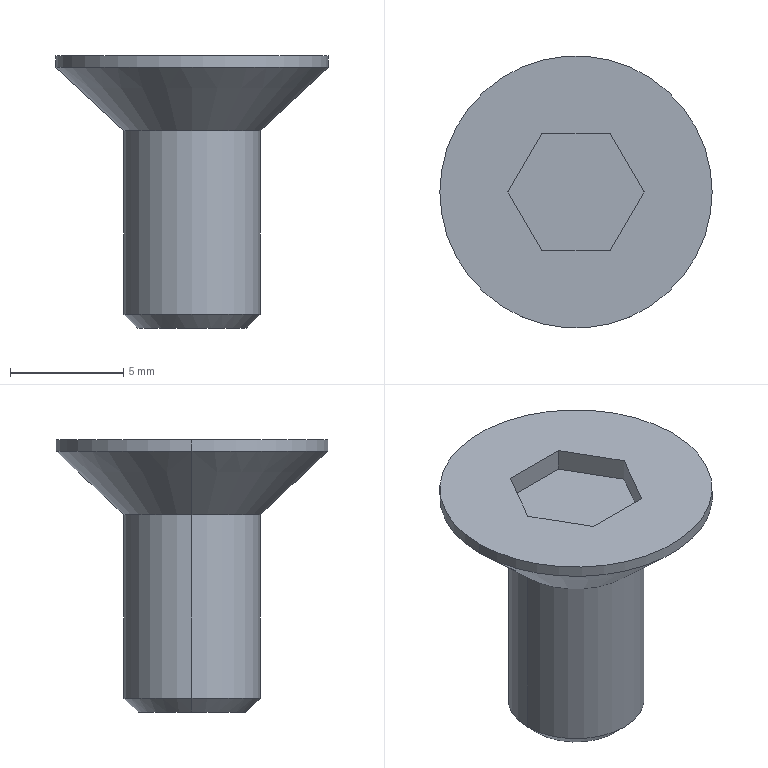Part | SolidWorks | features Chamfer 1, ICE 1, Revolution 1 | 1 solid | 17 faces | box 12 x 12 x 12 mm | volume 460.573 mm3 | plane 9 | cone 4 | cylinder 4 | commonest cylinder face diameters 6 x2 12 x2
STEP:
#1=CARTESIAN_POINT('',(-2.386,0.,-12.));
#2=VERTEX_POINT('',#1);
#3=CARTESIAN_POINT('',(2.386,0.,-12.));
#4=VERTEX_POINT('',#3);
#5=CARTESIAN_POINT('',(0.,0.,-12.));
#6=DIRECTION('',(0.,0.,-1.));
#7=DIRECTION('',(-1.,0.,0.));
#8=AXIS2_PLACEMENT_3D('',#5,#6,#7);
#9=CIRCLE('',#8,2.386);
#10=EDGE_CURVE('',#2,#4,#9,.T.);
#11=ORIENTED_EDGE('',*,*,#10,.F.);
#12=CARTESIAN_POINT('',(-3.,0.,-11.387));
#13=VERTEX_POINT('',#12);
#14=CARTESIAN_POINT('',(-3.,0.,-11.387));
#15=DIRECTION('',(-0.7071,0.,0.7071));
#16=VECTOR('',#15,1000.);
#17=LINE('',#14,#16);
#18=EDGE_CURVE('',#2,#13,#17,.T.);
#19=ORIENTED_EDGE('',*,*,#18,.T.);
#20=CARTESIAN_POINT('',(3.,0.,-11.387));
#21=VERTEX_POINT('',#20);
#22=CARTESIAN_POINT('',(0.,0.,-11.387));
#23=DIRECTION('',(0.,0.,1.));
#24=DIRECTION('',(-1.,0.,0.));
#25=AXIS2_PLACEMENT_3D('',#22,#23,#24);
#26=CIRCLE('',#25,3.);
#27=EDGE_CURVE('',#21,#13,#26,.T.);
#28=ORIENTED_EDGE('',*,*,#27,.F.);
#29=CARTESIAN_POINT('',(3.,0.,-11.387));
#30=DIRECTION('',(0.7071,0.,0.7071));
#31=VECTOR('',#30,1000.);
#32=LINE('',#29,#31);
#33=EDGE_CURVE('',#4,#21,#32,.T.);
#34=ORIENTED_EDGE('',*,*,#33,.F.);
#35=EDGE_LOOP('',(#11,#19,#28,#34));
#36=FACE_OUTER_BOUND('',#35,.T.);
#37=CARTESIAN_POINT('',(0.,0.,-11.387));
#38=DIRECTION('',(0.,0.,1.));
#39=DIRECTION('',(1.,0.,0.));
#40=AXIS2_PLACEMENT_3D('',#37,#38,#39);
#41=CONICAL_SURFACE('',#40,3.,0.7854);
#42=ADVANCED_FACE('',(#36),#41,.T.);
#43=CARTESIAN_POINT('',(3.,0.,-3.3));
#44=VERTEX_POINT('',#43);
#45=CARTESIAN_POINT('',(-3.,0.,-3.3));
#46=VERTEX_POINT('',#45);
#47=CARTESIAN_POINT('',(0.,0.,-3.3));
#48=DIRECTION('',(0.,0.,1.));
#49=DIRECTION('',(1.,0.,0.));
#50=AXIS2_PLACEMENT_3D('',#47,#48,#49);
#51=CIRCLE('',#50,3.);
#52=EDGE_CURVE('',#44,#46,#51,.T.);
#53=ORIENTED_EDGE('',*,*,#52,.T.);
#54=CARTESIAN_POINT('',(-6.,0.,-0.5));
#55=VERTEX_POINT('',#54);
#56=CARTESIAN_POINT('',(-6.,0.,-0.5));
#57=DIRECTION('',(-0.7311,0.,0.6823));
#58=VECTOR('',#57,1000.);
#59=LINE('',#56,#58);
#60=EDGE_CURVE('',#46,#55,#59,.T.);
#61=ORIENTED_EDGE('',*,*,#60,.T.);
#62=CARTESIAN_POINT('',(6.,0.,-0.5));
#63=VERTEX_POINT('',#62);
#64=CARTESIAN_POINT('',(0.,0.,-0.5));
#65=DIRECTION('',(0.,0.,1.));
#66=DIRECTION('',(1.,0.,0.));
#67=AXIS2_PLACEMENT_3D('',#64,#65,#66);
#68=CIRCLE('',#67,6.);
#69=EDGE_CURVE('',#63,#55,#68,.T.);
#70=ORIENTED_EDGE('',*,*,#69,.F.);
#71=CARTESIAN_POINT('',(6.,0.,-0.5));
#72=DIRECTION('',(0.7311,0.,0.6823));
#73=VECTOR('',#72,1000.);
#74=LINE('',#71,#73);
#75=EDGE_CURVE('',#44,#63,#74,.T.);
#76=ORIENTED_EDGE('',*,*,#75,.F.);
#77=EDGE_LOOP('',(#53,#61,#70,#76));
#78=FACE_OUTER_BOUND('',#77,.T.);
#79=CARTESIAN_POINT('',(0.,0.,-0.5));
#80=DIRECTION('',(0.,0.,1.));
#81=DIRECTION('',(1.,0.,0.));
#82=AXIS2_PLACEMENT_3D('',#79,#80,#81);
#83=CONICAL_SURFACE('',#82,6.,0.8199);
#84=ADVANCED_FACE('',(#78),#83,.T.);
#85=ORIENTED_EDGE('',*,*,#69,.T.);
#86=CARTESIAN_POINT('',(-6.,0.,0.));
#87=VERTEX_POINT('',#86);
#88=CARTESIAN_POINT('',(-6.,0.,-12.));
#89=DIRECTION('',(0.,0.,1.));
#90=VECTOR('',#89,1000.);
#91=LINE('',#88,#90);
#92=EDGE_CURVE('',#55,#87,#91,.T.);
#93=ORIENTED_EDGE('',*,*,#92,.T.);
#94=CARTESIAN_POINT('',(6.,0.,0.));
#95=VERTEX_POINT('',#94);
#96=CARTESIAN_POINT('',(0.,0.,0.));
#97=DIRECTION('',(0.,0.,1.));
#98=DIRECTION('',(1.,0.,0.));
#99=AXIS2_PLACEMENT_3D('',#96,#97,#98);
#100=CIRCLE('',#99,6.);
#101=EDGE_CURVE('',#95,#87,#100,.T.);
#102=ORIENTED_EDGE('',*,*,#101,.F.);
#103=CARTESIAN_POINT('',(6.,0.,-12.));
#104=DIRECTION('',(0.,0.,1.));
#105=VECTOR('',#104,1000.);
#106=LINE('',#103,#105);
#107=EDGE_CURVE('',#63,#95,#106,.T.);
#108=ORIENTED_EDGE('',*,*,#107,.F.);
#109=EDGE_LOOP('',(#85,#93,#102,#108));
#110=FACE_OUTER_BOUND('',#109,.T.);
#111=CARTESIAN_POINT('',(0.,0.,-12.));
#112=DIRECTION('',(0.,0.,1.));
#113=DIRECTION('',(1.,0.,0.));
#114=AXIS2_PLACEMENT_3D('',#111,#112,#113);
#115=CYLINDRICAL_SURFACE('',#114,6.);
#116=ADVANCED_FACE('',(#110),#115,.T.);
#117=ORIENTED_EDGE('',*,*,#27,.T.);
#118=CARTESIAN_POINT('',(-3.,0.,-12.));
#119=DIRECTION('',(0.,0.,1.));
#120=VECTOR('',#119,1000.);
#121=LINE('',#118,#120);
#122=EDGE_CURVE('',#13,#46,#121,.T.);
#123=ORIENTED_EDGE('',*,*,#122,.T.);
#124=ORIENTED_EDGE('',*,*,#52,.F.);
#125=CARTESIAN_POINT('',(3.,0.,-12.));
#126=DIRECTION('',(0.,0.,1.));
#127=VECTOR('',#126,1000.);
#128=LINE('',#125,#127);
#129=EDGE_CURVE('',#21,#44,#128,.T.);
#130=ORIENTED_EDGE('',*,*,#129,.F.);
#131=EDGE_LOOP('',(#117,#123,#124,#130));
#132=FACE_OUTER_BOUND('',#131,.T.);
#133=CARTESIAN_POINT('',(0.,0.,-12.));
#134=DIRECTION('',(0.,0.,1.));
#135=DIRECTION('',(1.,0.,0.));
#136=AXIS2_PLACEMENT_3D('',#133,#134,#135);
#137=CYLINDRICAL_SURFACE('',#136,3.);
#138=ADVANCED_FACE('',(#132),#137,.T.);
#139=ORIENTED_EDGE('',*,*,#122,.F.);
#140=CARTESIAN_POINT('',(0.,0.,-11.387));
#141=DIRECTION('',(0.,0.,1.));
#142=DIRECTION('',(-1.,0.,0.));
#143=AXIS2_PLACEMENT_3D('',#140,#141,#142);
#144=CIRCLE('',#143,3.);
#145=EDGE_CURVE('',#13,#21,#144,.T.);
#146=ORIENTED_EDGE('',*,*,#145,.T.);
#147=ORIENTED_EDGE('',*,*,#129,.T.);
#148=CARTESIAN_POINT('',(0.,0.,-3.3));
#149=DIRECTION('',(0.,0.,1.));
#150=DIRECTION('',(1.,0.,0.));
#151=AXIS2_PLACEMENT_3D('',#148,#149,#150);
#152=CIRCLE('',#151,3.);
#153=EDGE_CURVE('',#46,#44,#152,.T.);
#154=ORIENTED_EDGE('',*,*,#153,.F.);
#155=EDGE_LOOP('',(#139,#146,#147,#154));
#156=FACE_OUTER_BOUND('',#155,.T.);
#157=CARTESIAN_POINT('',(0.,0.,-12.));
#158=DIRECTION('',(0.,0.,1.));
#159=DIRECTION('',(1.,0.,0.));
#160=AXIS2_PLACEMENT_3D('',#157,#158,#159);
#161=CYLINDRICAL_SURFACE('',#160,3.);
#162=ADVANCED_FACE('',(#156),#161,.T.);
#163=CARTESIAN_POINT('',(0.,0.,-12.));
#164=DIRECTION('',(0.,0.,-1.));
#165=DIRECTION('',(-1.,0.,0.));
#166=AXIS2_PLACEMENT_3D('',#163,#164,#165);
#167=CIRCLE('',#166,2.386);
#168=EDGE_CURVE('',#4,#2,#167,.T.);
#169=ORIENTED_EDGE('',*,*,#168,.T.);
#170=ORIENTED_EDGE('',*,*,#10,.T.);
#171=EDGE_LOOP('',(#169,#170));
#172=FACE_OUTER_BOUND('',#171,.T.);
#173=CARTESIAN_POINT('',(3.,0.,-12.));
#174=DIRECTION('',(0.,0.,-1.));
#175=DIRECTION('',(-1.,0.,0.));
#176=AXIS2_PLACEMENT_3D('',#173,#174,#175);
#177=PLANE('',#176);
#178=ADVANCED_FACE('',(#172),#177,.T.);
#179=CARTESIAN_POINT('',(-1.5,-2.598,0.));
#180=VERTEX_POINT('',#179);
#181=CARTESIAN_POINT('',(1.5,-2.598,0.));
#182=VERTEX_POINT('',#181);
#183=CARTESIAN_POINT('',(-1.5,-2.598,0.));
#184=DIRECTION('',(1.,0.,0.));
#185=VECTOR('',#184,1000.);
#186=LINE('',#183,#185);
#187=EDGE_CURVE('',#180,#182,#186,.T.);
#188=ORIENTED_EDGE('',*,*,#187,.F.);
#189=CARTESIAN_POINT('',(-3.,0.,0.));
#190=VERTEX_POINT('',#189);
#191=CARTESIAN_POINT('',(-3.,0.,0.));
#192=DIRECTION('',(0.5,-0.866,0.));
#193=VECTOR('',#192,1000.);
#194=LINE('',#191,#193);
#195=EDGE_CURVE('',#190,#180,#194,.T.);
#196=ORIENTED_EDGE('',*,*,#195,.F.);
#197=CARTESIAN_POINT('',(-1.5,2.598,0.));
#198=VERTEX_POINT('',#197);
#199=CARTESIAN_POINT('',(-1.5,2.598,0.));
#200=DIRECTION('',(-0.5,-0.866,0.));
#201=VECTOR('',#200,1000.);
#202=LINE('',#199,#201);
#203=EDGE_CURVE('',#198,#190,#202,.T.);
#204=ORIENTED_EDGE('',*,*,#203,.F.);
#205=CARTESIAN_POINT('',(1.5,2.598,0.));
#206=VERTEX_POINT('',#205);
#207=CARTESIAN_POINT('',(1.5,2.598,0.));
#208=DIRECTION('',(-1.,0.,0.));
#209=VECTOR('',#208,1000.);
#210=LINE('',#207,#209);
#211=EDGE_CURVE('',#206,#198,#210,.T.);
#212=ORIENTED_EDGE('',*,*,#211,.F.);
#213=CARTESIAN_POINT('',(3.,0.,0.));
#214=VERTEX_POINT('',#213);
#215=CARTESIAN_POINT('',(3.,0.,0.));
#216=DIRECTION('',(-0.5,0.866,0.));
#217=VECTOR('',#216,1000.);
#218=LINE('',#215,#217);
#219=EDGE_CURVE('',#214,#206,#218,.T.);
#220=ORIENTED_EDGE('',*,*,#219,.F.);
#221=CARTESIAN_POINT('',(1.5,-2.598,0.));
#222=DIRECTION('',(0.5,0.866,0.));
#223=VECTOR('',#222,1000.);
#224=LINE('',#221,#223);
#225=EDGE_CURVE('',#182,#214,#224,.T.);
#226=ORIENTED_EDGE('',*,*,#225,.F.);
#227=EDGE_LOOP('',(#188,#196,#204,#212,#220,#226));
#228=FACE_BOUND('',#227,.T.);
#229=ORIENTED_EDGE('',*,*,#101,.T.);
#230=CARTESIAN_POINT('',(0.,0.,0.));
#231=DIRECTION('',(0.,0.,1.));
#232=DIRECTION('',(1.,0.,0.));
#233=AXIS2_PLACEMENT_3D('',#230,#231,#232);
#234=CIRCLE('',#233,6.);
#235=EDGE_CURVE('',#87,#95,#234,.T.);
#236=ORIENTED_EDGE('',*,*,#235,.T.);
#237=EDGE_LOOP('',(#229,#236));
#238=FACE_OUTER_BOUND('',#237,.T.);
#239=CARTESIAN_POINT('',(0.,0.,0.));
#240=DIRECTION('',(0.,0.,1.));
#241=DIRECTION('',(1.,0.,0.));
#242=AXIS2_PLACEMENT_3D('',#239,#240,#241);
#243=PLANE('',#242);
#244=ADVANCED_FACE('',(#228,#238),#243,.T.);
#245=ORIENTED_EDGE('',*,*,#92,.F.);
#246=CARTESIAN_POINT('',(0.,0.,-0.5));
#247=DIRECTION('',(0.,0.,1.));
#248=DIRECTION('',(1.,0.,0.));
#249=AXIS2_PLACEMENT_3D('',#246,#247,#248);
#250=CIRCLE('',#249,6.);
#251=EDGE_CURVE('',#55,#63,#250,.T.);
#252=ORIENTED_EDGE('',*,*,#251,.T.);
#253=ORIENTED_EDGE('',*,*,#107,.T.);
#254=ORIENTED_EDGE('',*,*,#235,.F.);
#255=EDGE_LOOP('',(#245,#252,#253,#254));
#256=FACE_OUTER_BOUND('',#255,.T.);
#257=CARTESIAN_POINT('',(0.,0.,-12.));
#258=DIRECTION('',(0.,0.,1.));
#259=DIRECTION('',(1.,0.,0.));
#260=AXIS2_PLACEMENT_3D('',#257,#258,#259);
#261=CYLINDRICAL_SURFACE('',#260,6.);
#262=ADVANCED_FACE('',(#256),#261,.T.);
#263=ORIENTED_EDGE('',*,*,#60,.F.);
#264=ORIENTED_EDGE('',*,*,#153,.T.);
#265=ORIENTED_EDGE('',*,*,#75,.T.);
#266=ORIENTED_EDGE('',*,*,#251,.F.);
#267=EDGE_LOOP('',(#263,#264,#265,#266));
#268=FACE_OUTER_BOUND('',#267,.T.);
#269=CARTESIAN_POINT('',(0.,0.,-0.5));
#270=DIRECTION('',(0.,0.,1.));
#271=DIRECTION('',(1.,0.,0.));
#272=AXIS2_PLACEMENT_3D('',#269,#270,#271);
#273=CONICAL_SURFACE('',#272,6.,0.8199);
#274=ADVANCED_FACE('',(#268),#273,.T.);
#275=ORIENTED_EDGE('',*,*,#187,.T.);
#276=CARTESIAN_POINT('',(1.5,-2.598,-1.));
#277=VERTEX_POINT('',#276);
#278=CARTESIAN_POINT('',(1.5,-2.598,-1.));
#279=DIRECTION('',(0.,0.,1.));
#280=VECTOR('',#279,1000.);
#281=LINE('',#278,#280);
#282=EDGE_CURVE('',#277,#182,#281,.T.);
#283=ORIENTED_EDGE('',*,*,#282,.F.);
#284=CARTESIAN_POINT('',(-1.5,-2.598,-1.));
#285=VERTEX_POINT('',#284);
#286=CARTESIAN_POINT('',(-1.5,-2.598,-1.));
#287=DIRECTION('',(1.,0.,0.));
#288=VECTOR('',#287,1000.);
#289=LINE('',#286,#288);
#290=EDGE_CURVE('',#285,#277,#289,.T.);
#291=ORIENTED_EDGE('',*,*,#290,.F.);
#292=CARTESIAN_POINT('',(-1.5,-2.598,-1.));
#293=DIRECTION('',(0.,0.,1.));
#294=VECTOR('',#293,1000.);
#295=LINE('',#292,#294);
#296=EDGE_CURVE('',#285,#180,#295,.T.);
#297=ORIENTED_EDGE('',*,*,#296,.T.);
#298=EDGE_LOOP('',(#275,#283,#291,#297));
#299=FACE_OUTER_BOUND('',#298,.T.);
#300=CARTESIAN_POINT('',(-1.5,-2.598,-1.));
#301=DIRECTION('',(0.,-1.,0.));
#302=DIRECTION('',(1.,0.,0.));
#303=AXIS2_PLACEMENT_3D('',#300,#301,#302);
#304=PLANE('',#303);
#305=ADVANCED_FACE('',(#299),#304,.F.);
#306=ORIENTED_EDGE('',*,*,#195,.T.);
#307=ORIENTED_EDGE('',*,*,#296,.F.);
#308=CARTESIAN_POINT('',(-3.,0.,-1.));
#309=VERTEX_POINT('',#308);
#310=CARTESIAN_POINT('',(-3.,0.,-1.));
#311=DIRECTION('',(0.5,-0.866,0.));
#312=VECTOR('',#311,1000.);
#313=LINE('',#310,#312);
#314=EDGE_CURVE('',#309,#285,#313,.T.);
#315=ORIENTED_EDGE('',*,*,#314,.F.);
#316=CARTESIAN_POINT('',(-3.,0.,-1.));
#317=DIRECTION('',(0.,0.,1.));
#318=VECTOR('',#317,1000.);
#319=LINE('',#316,#318);
#320=EDGE_CURVE('',#309,#190,#319,.T.);
#321=ORIENTED_EDGE('',*,*,#320,.T.);
#322=EDGE_LOOP('',(#306,#307,#315,#321));
#323=FACE_OUTER_BOUND('',#322,.T.);
#324=CARTESIAN_POINT('',(-3.,0.,-1.));
#325=DIRECTION('',(-0.866,-0.5,0.));
#326=DIRECTION('',(0.5,-0.866,0.));
#327=AXIS2_PLACEMENT_3D('',#324,#325,#326);
#328=PLANE('',#327);
#329=ADVANCED_FACE('',(#323),#328,.F.);
#330=ORIENTED_EDGE('',*,*,#203,.T.);
#331=ORIENTED_EDGE('',*,*,#320,.F.);
#332=CARTESIAN_POINT('',(-1.5,2.598,-1.));
#333=VERTEX_POINT('',#332);
#334=CARTESIAN_POINT('',(-1.5,2.598,-1.));
#335=DIRECTION('',(-0.5,-0.866,0.));
#336=VECTOR('',#335,1000.);
#337=LINE('',#334,#336);
#338=EDGE_CURVE('',#333,#309,#337,.T.);
#339=ORIENTED_EDGE('',*,*,#338,.F.);
#340=CARTESIAN_POINT('',(-1.5,2.598,-1.));
#341=DIRECTION('',(0.,0.,1.));
#342=VECTOR('',#341,1000.);
#343=LINE('',#340,#342);
#344=EDGE_CURVE('',#333,#198,#343,.T.);
#345=ORIENTED_EDGE('',*,*,#344,.T.);
#346=EDGE_LOOP('',(#330,#331,#339,#345));
#347=FACE_OUTER_BOUND('',#346,.T.);
#348=CARTESIAN_POINT('',(-1.5,2.598,-1.));
#349=DIRECTION('',(-0.866,0.5,0.));
#350=DIRECTION('',(-0.5,-0.866,0.));
#351=AXIS2_PLACEMENT_3D('',#348,#349,#350);
#352=PLANE('',#351);
#353=ADVANCED_FACE('',(#347),#352,.F.);
#354=ORIENTED_EDGE('',*,*,#211,.T.);
#355=ORIENTED_EDGE('',*,*,#344,.F.);
#356=CARTESIAN_POINT('',(1.5,2.598,-1.));
#357=VERTEX_POINT('',#356);
#358=CARTESIAN_POINT('',(1.5,2.598,-1.));
#359=DIRECTION('',(-1.,0.,0.));
#360=VECTOR('',#359,1000.);
#361=LINE('',#358,#360);
#362=EDGE_CURVE('',#357,#333,#361,.T.);
#363=ORIENTED_EDGE('',*,*,#362,.F.);
#364=CARTESIAN_POINT('',(1.5,2.598,-1.));
#365=DIRECTION('',(0.,0.,1.));
#366=VECTOR('',#365,1000.);
#367=LINE('',#364,#366);
#368=EDGE_CURVE('',#357,#206,#367,.T.);
#369=ORIENTED_EDGE('',*,*,#368,.T.);
#370=EDGE_LOOP('',(#354,#355,#363,#369));
#371=FACE_OUTER_BOUND('',#370,.T.);
#372=CARTESIAN_POINT('',(1.5,2.598,-1.));
#373=DIRECTION('',(0.,1.,0.));
#374=DIRECTION('',(0.,0.,1.));
#375=AXIS2_PLACEMENT_3D('',#372,#373,#374);
#376=PLANE('',#375);
#377=ADVANCED_FACE('',(#371),#376,.F.);
#378=ORIENTED_EDGE('',*,*,#219,.T.);
#379=ORIENTED_EDGE('',*,*,#368,.F.);
#380=CARTESIAN_POINT('',(3.,0.,-1.));
#381=VERTEX_POINT('',#380);
#382=CARTESIAN_POINT('',(3.,0.,-1.));
#383=DIRECTION('',(-0.5,0.866,0.));
#384=VECTOR('',#383,1000.);
#385=LINE('',#382,#384);
#386=EDGE_CURVE('',#381,#357,#385,.T.);
#387=ORIENTED_EDGE('',*,*,#386,.F.);
#388=CARTESIAN_POINT('',(3.,0.,-1.));
#389=DIRECTION('',(0.,0.,1.));
#390=VECTOR('',#389,1000.);
#391=LINE('',#388,#390);
#392=EDGE_CURVE('',#381,#214,#391,.T.);
#393=ORIENTED_EDGE('',*,*,#392,.T.);
#394=EDGE_LOOP('',(#378,#379,#387,#393));
#395=FACE_OUTER_BOUND('',#394,.T.);
#396=CARTESIAN_POINT('',(3.,0.,-1.));
#397=DIRECTION('',(0.866,0.5,0.));
#398=DIRECTION('',(-0.5,0.866,0.));
#399=AXIS2_PLACEMENT_3D('',#396,#397,#398);
#400=PLANE('',#399);
#401=ADVANCED_FACE('',(#395),#400,.F.);
#402=ORIENTED_EDGE('',*,*,#225,.T.);
#403=ORIENTED_EDGE('',*,*,#392,.F.);
#404=CARTESIAN_POINT('',(1.5,-2.598,-1.));
#405=DIRECTION('',(0.5,0.866,0.));
#406=VECTOR('',#405,1000.);
#407=LINE('',#404,#406);
#408=EDGE_CURVE('',#277,#381,#407,.T.);
#409=ORIENTED_EDGE('',*,*,#408,.F.);
#410=ORIENTED_EDGE('',*,*,#282,.T.);
#411=EDGE_LOOP('',(#402,#403,#409,#410));
#412=FACE_OUTER_BOUND('',#411,.T.);
#413=CARTESIAN_POINT('',(1.5,-2.598,-1.));
#414=DIRECTION('',(0.866,-0.5,0.));
#415=DIRECTION('',(0.5,0.866,0.));
#416=AXIS2_PLACEMENT_3D('',#413,#414,#415);
#417=PLANE('',#416);
#418=ADVANCED_FACE('',(#412),#417,.F.);
#419=ORIENTED_EDGE('',*,*,#290,.T.);
#420=ORIENTED_EDGE('',*,*,#408,.T.);
#421=ORIENTED_EDGE('',*,*,#386,.T.);
#422=ORIENTED_EDGE('',*,*,#362,.T.);
#423=ORIENTED_EDGE('',*,*,#338,.T.);
#424=ORIENTED_EDGE('',*,*,#314,.T.);
#425=EDGE_LOOP('',(#419,#420,#421,#422,#423,#424));
#426=FACE_OUTER_BOUND('',#425,.T.);
#427=CARTESIAN_POINT('',(0.,0.,-1.));
#428=DIRECTION('',(0.,0.,1.));
#429=DIRECTION('',(1.,0.,0.));
#430=AXIS2_PLACEMENT_3D('',#427,#428,#429);
#431=PLANE('',#430);
#432=ADVANCED_FACE('',(#426),#431,.T.);
#433=ORIENTED_EDGE('',*,*,#18,.F.);
#434=ORIENTED_EDGE('',*,*,#168,.F.);
#435=ORIENTED_EDGE('',*,*,#33,.T.);
#436=ORIENTED_EDGE('',*,*,#145,.F.);
#437=EDGE_LOOP('',(#433,#434,#435,#436));
#438=FACE_OUTER_BOUND('',#437,.T.);
#439=CARTESIAN_POINT('',(0.,0.,-11.387));
#440=DIRECTION('',(0.,0.,1.));
#441=DIRECTION('',(1.,0.,0.));
#442=AXIS2_PLACEMENT_3D('',#439,#440,#441);
#443=CONICAL_SURFACE('',#442,3.,0.7854);
#444=ADVANCED_FACE('',(#438),#443,.T.);
#445=CLOSED_SHELL('',(#42,#84,#116,#138,#162,#178,#244,#262,#274,#305,#329,#353,#377,#401,#418,#432,#444));
#446=MANIFOLD_SOLID_BREP('',#445);
#447=CARTESIAN_POINT('',(0.,0.,0.));
#448=DIRECTION('',(0.,0.,1.));
#449=DIRECTION('',(1.,0.,0.));
#450=AXIS2_PLACEMENT_3D('',#447,#448,#449);
#451=(LENGTH_UNIT()NAMED_UNIT(*)SI_UNIT(.MILLI.,.METRE.));
#452=UNCERTAINTY_MEASURE_WITH_UNIT(LENGTH_MEASURE(0.00001),#451,'','');
#453=(NAMED_UNIT(*)PLANE_ANGLE_UNIT()SI_UNIT($,.RADIAN.));
#454=(NAMED_UNIT(*)SI_UNIT($,.STERADIAN.)SOLID_ANGLE_UNIT());
#455=(GEOMETRIC_REPRESENTATION_CONTEXT(3)GLOBAL_UNCERTAINTY_ASSIGNED_CONTEXT((#452))GLOBAL_UNIT_ASSIGNED_CONTEXT((#451,#453,#454))REPRESENTATION_CONTEXT('',''));
#456=ADVANCED_BREP_SHAPE_REPRESENTATION('',(#446,#450),#455);